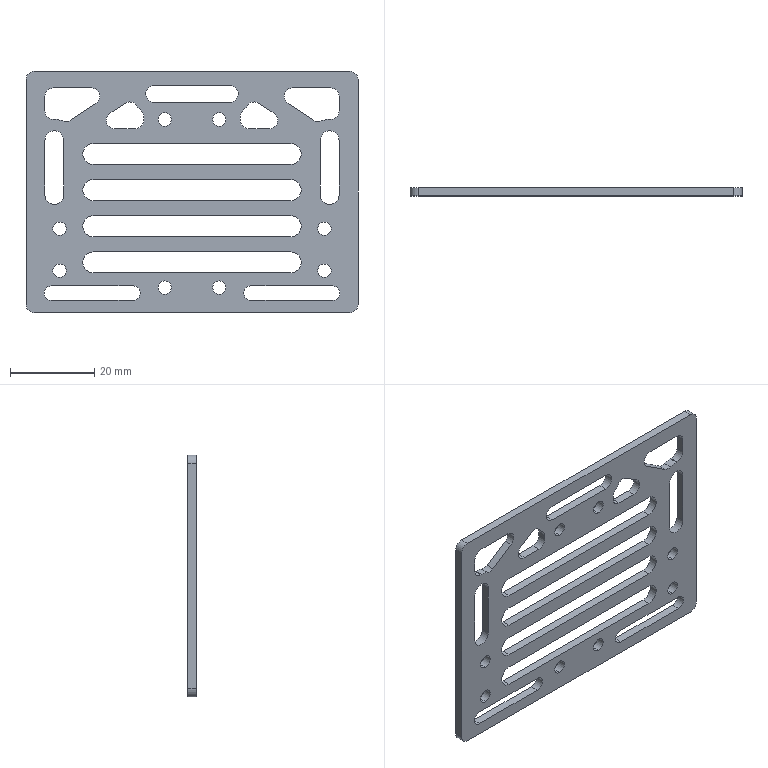Part | SolidWorks | features Extrusion 1, Fillet 1, ICE 1 | 1 solid | 100 faces | box 79 x 2 x 57.5 mm | volume 5646 mm3 | cylinder 64 | plane 36 | commonest cylinder face diameters 4 x24 3.2 x16 5 x8 4.5 x6 10 x6 3.4 x4